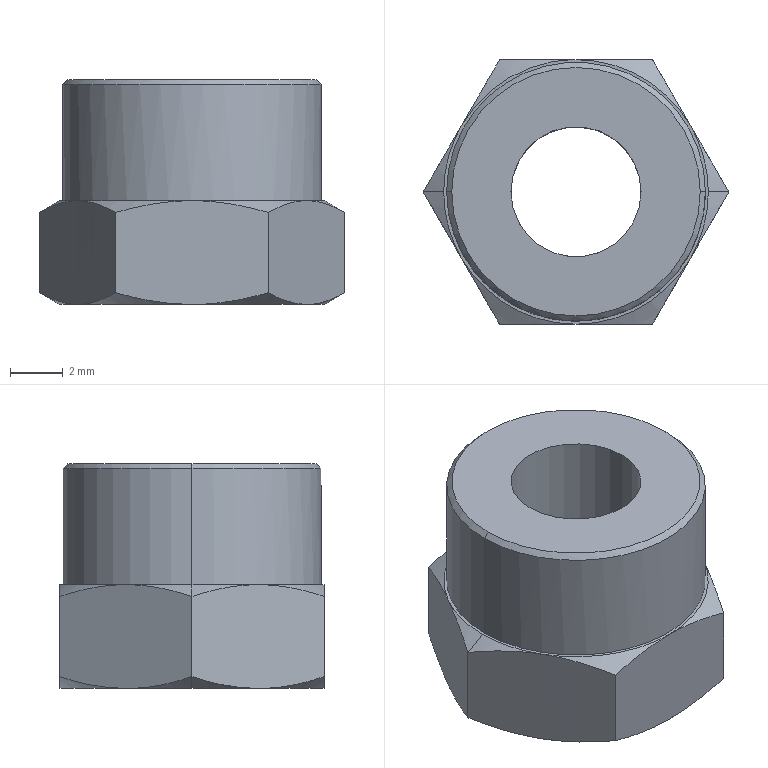Part | STEP file | 46A-01002LM15_Default<As Machined> | 1 solid | 67 faces | box 11.547 x 10 x 8.5 mm | volume 503.163 mm3 | cone 44 | cylinder 14 | plane 9 | commonest cylinder face diameters 4.917 x12 9.78 x2